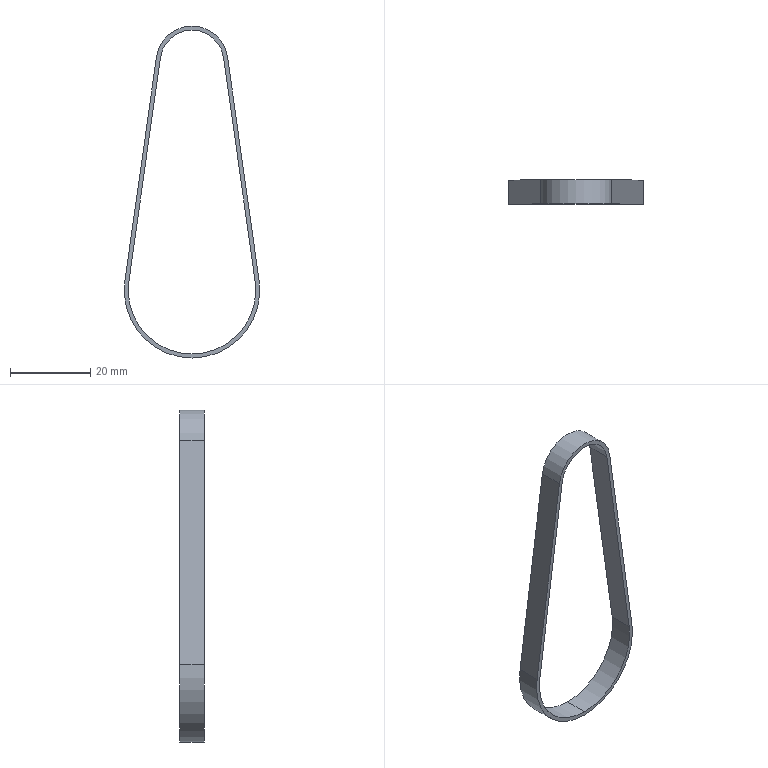Part | SolidWorks | features Extrusion 1 | 1 solid | 12 faces | box 33.828 x 6 x 82.868 mm | volume 1159 mm3 | cylinder 6 | plane 6 | commonest cylinder face diameters 31.828 x2 33.828 x2 15.908 x1 17.908 x1
STEP:
#1=CARTESIAN_POINT('',(15.758,6.,-54.778));
#2=VERTEX_POINT('',#1);
#3=CARTESIAN_POINT('',(0.,6.,-72.914));
#4=VERTEX_POINT('',#3);
#5=CARTESIAN_POINT('',(0.,6.,-57.));
#6=DIRECTION('',(0.,1.,0.));
#7=DIRECTION('',(0.,0.,1.));
#8=AXIS2_PLACEMENT_3D('',#5,#6,#7);
#9=CIRCLE('',#8,15.914);
#10=EDGE_CURVE('',#2,#4,#9,.T.);
#11=ORIENTED_EDGE('',*,*,#10,.T.);
#12=CARTESIAN_POINT('',(0.,0.,-72.914));
#13=VERTEX_POINT('',#12);
#14=CARTESIAN_POINT('',(0.,6.,-72.914));
#15=DIRECTION('',(0.,-1.,0.));
#16=VECTOR('',#15,1000.);
#17=LINE('',#14,#16);
#18=EDGE_CURVE('',#4,#13,#17,.T.);
#19=ORIENTED_EDGE('',*,*,#18,.T.);
#20=CARTESIAN_POINT('',(15.758,0.,-54.778));
#21=VERTEX_POINT('',#20);
#22=CARTESIAN_POINT('',(0.,0.,-57.));
#23=DIRECTION('',(0.,1.,0.));
#24=DIRECTION('',(0.,0.,1.));
#25=AXIS2_PLACEMENT_3D('',#22,#23,#24);
#26=CIRCLE('',#25,15.914);
#27=EDGE_CURVE('',#21,#13,#26,.T.);
#28=ORIENTED_EDGE('',*,*,#27,.F.);
#29=CARTESIAN_POINT('',(15.758,6.,-54.778));
#30=DIRECTION('',(0.,-1.,0.));
#31=VECTOR('',#30,1000.);
#32=LINE('',#29,#31);
#33=EDGE_CURVE('',#2,#21,#32,.T.);
#34=ORIENTED_EDGE('',*,*,#33,.F.);
#35=EDGE_LOOP('',(#11,#19,#28,#34));
#36=FACE_OUTER_BOUND('',#35,.T.);
#37=CARTESIAN_POINT('',(0.,6.,-57.));
#38=DIRECTION('',(0.,-1.,0.));
#39=DIRECTION('',(0.,0.,-1.));
#40=AXIS2_PLACEMENT_3D('',#37,#38,#39);
#41=CYLINDRICAL_SURFACE('',#40,15.914);
#42=ADVANCED_FACE('',(#36),#41,.F.);
#43=CARTESIAN_POINT('',(0.,6.,-73.914));
#44=VERTEX_POINT('',#43);
#45=CARTESIAN_POINT('',(-16.748,6.,-54.638));
#46=VERTEX_POINT('',#45);
#47=CARTESIAN_POINT('',(0.,6.,-57.));
#48=DIRECTION('',(0.,1.,0.));
#49=DIRECTION('',(0.,0.,1.));
#50=AXIS2_PLACEMENT_3D('',#47,#48,#49);
#51=CIRCLE('',#50,16.914);
#52=EDGE_CURVE('',#44,#46,#51,.T.);
#53=ORIENTED_EDGE('',*,*,#52,.F.);
#54=CARTESIAN_POINT('',(0.,0.,-73.914));
#55=VERTEX_POINT('',#54);
#56=CARTESIAN_POINT('',(0.,6.,-73.914));
#57=DIRECTION('',(0.,-1.,0.));
#58=VECTOR('',#57,1000.);
#59=LINE('',#56,#58);
#60=EDGE_CURVE('',#44,#55,#59,.T.);
#61=ORIENTED_EDGE('',*,*,#60,.T.);
#62=CARTESIAN_POINT('',(-16.748,0.,-54.638));
#63=VERTEX_POINT('',#62);
#64=CARTESIAN_POINT('',(0.,0.,-57.));
#65=DIRECTION('',(0.,1.,0.));
#66=DIRECTION('',(0.,0.,1.));
#67=AXIS2_PLACEMENT_3D('',#64,#65,#66);
#68=CIRCLE('',#67,16.914);
#69=EDGE_CURVE('',#55,#63,#68,.T.);
#70=ORIENTED_EDGE('',*,*,#69,.T.);
#71=CARTESIAN_POINT('',(-16.748,6.,-54.638));
#72=DIRECTION('',(0.,-1.,0.));
#73=VECTOR('',#72,1000.);
#74=LINE('',#71,#73);
#75=EDGE_CURVE('',#46,#63,#74,.T.);
#76=ORIENTED_EDGE('',*,*,#75,.F.);
#77=EDGE_LOOP('',(#53,#61,#70,#76));
#78=FACE_OUTER_BOUND('',#77,.T.);
#79=CARTESIAN_POINT('',(0.,6.,-57.));
#80=DIRECTION('',(0.,-1.,0.));
#81=DIRECTION('',(0.,0.,-1.));
#82=AXIS2_PLACEMENT_3D('',#79,#80,#81);
#83=CYLINDRICAL_SURFACE('',#82,16.914);
#84=ADVANCED_FACE('',(#78),#83,.T.);
#85=CARTESIAN_POINT('',(16.748,6.,-54.638));
#86=VERTEX_POINT('',#85);
#87=CARTESIAN_POINT('',(0.,6.,-57.));
#88=DIRECTION('',(0.,1.,0.));
#89=DIRECTION('',(0.,0.,1.));
#90=AXIS2_PLACEMENT_3D('',#87,#88,#89);
#91=CIRCLE('',#90,16.914);
#92=EDGE_CURVE('',#86,#44,#91,.T.);
#93=ORIENTED_EDGE('',*,*,#92,.T.);
#94=ORIENTED_EDGE('',*,*,#52,.T.);
#95=CARTESIAN_POINT('',(-8.866,6.,1.25));
#96=VERTEX_POINT('',#95);
#97=CARTESIAN_POINT('',(-16.748,6.,-54.638));
#98=DIRECTION('',(0.1396,0.,0.9902));
#99=VECTOR('',#98,1000.);
#100=LINE('',#97,#99);
#101=EDGE_CURVE('',#46,#96,#100,.T.);
#102=ORIENTED_EDGE('',*,*,#101,.T.);
#103=CARTESIAN_POINT('',(8.866,6.,1.25));
#104=VERTEX_POINT('',#103);
#105=CARTESIAN_POINT('',(0.,6.,0.));
#106=DIRECTION('',(0.,1.,0.));
#107=DIRECTION('',(0.,0.,1.));
#108=AXIS2_PLACEMENT_3D('',#105,#106,#107);
#109=CIRCLE('',#108,8.954);
#110=EDGE_CURVE('',#96,#104,#109,.T.);
#111=ORIENTED_EDGE('',*,*,#110,.T.);
#112=CARTESIAN_POINT('',(16.748,6.,-54.638));
#113=DIRECTION('',(0.1396,0.,-0.9902));
#114=VECTOR('',#113,1000.);
#115=LINE('',#112,#114);
#116=EDGE_CURVE('',#104,#86,#115,.T.);
#117=ORIENTED_EDGE('',*,*,#116,.T.);
#118=EDGE_LOOP('',(#93,#94,#102,#111,#117));
#119=FACE_OUTER_BOUND('',#118,.T.);
#120=CARTESIAN_POINT('',(7.876,6.,1.111));
#121=VERTEX_POINT('',#120);
#122=CARTESIAN_POINT('',(15.758,6.,-54.778));
#123=DIRECTION('',(0.1396,0.,-0.9902));
#124=VECTOR('',#123,1000.);
#125=LINE('',#122,#124);
#126=EDGE_CURVE('',#121,#2,#125,.T.);
#127=ORIENTED_EDGE('',*,*,#126,.F.);
#128=CARTESIAN_POINT('',(-7.876,6.,1.111));
#129=VERTEX_POINT('',#128);
#130=CARTESIAN_POINT('',(0.,6.,0.));
#131=DIRECTION('',(0.,1.,0.));
#132=DIRECTION('',(0.,0.,1.));
#133=AXIS2_PLACEMENT_3D('',#130,#131,#132);
#134=CIRCLE('',#133,7.954);
#135=EDGE_CURVE('',#129,#121,#134,.T.);
#136=ORIENTED_EDGE('',*,*,#135,.F.);
#137=CARTESIAN_POINT('',(-15.758,6.,-54.778));
#138=VERTEX_POINT('',#137);
#139=CARTESIAN_POINT('',(-15.758,6.,-54.778));
#140=DIRECTION('',(0.1396,0.,0.9902));
#141=VECTOR('',#140,1000.);
#142=LINE('',#139,#141);
#143=EDGE_CURVE('',#138,#129,#142,.T.);
#144=ORIENTED_EDGE('',*,*,#143,.F.);
#145=CARTESIAN_POINT('',(0.,6.,-57.));
#146=DIRECTION('',(0.,1.,0.));
#147=DIRECTION('',(0.,0.,1.));
#148=AXIS2_PLACEMENT_3D('',#145,#146,#147);
#149=CIRCLE('',#148,15.914);
#150=EDGE_CURVE('',#4,#138,#149,.T.);
#151=ORIENTED_EDGE('',*,*,#150,.F.);
#152=ORIENTED_EDGE('',*,*,#10,.F.);
#153=EDGE_LOOP('',(#127,#136,#144,#151,#152));
#154=FACE_BOUND('',#153,.T.);
#155=CARTESIAN_POINT('',(0.,6.,-57.));
#156=DIRECTION('',(0.,1.,0.));
#157=DIRECTION('',(0.,0.,1.));
#158=AXIS2_PLACEMENT_3D('',#155,#156,#157);
#159=PLANE('',#158);
#160=ADVANCED_FACE('',(#119,#154),#159,.T.);
#161=CARTESIAN_POINT('',(16.748,0.,-54.638));
#162=VERTEX_POINT('',#161);
#163=CARTESIAN_POINT('',(0.,0.,-57.));
#164=DIRECTION('',(0.,1.,0.));
#165=DIRECTION('',(0.,0.,1.));
#166=AXIS2_PLACEMENT_3D('',#163,#164,#165);
#167=CIRCLE('',#166,16.914);
#168=EDGE_CURVE('',#162,#55,#167,.T.);
#169=ORIENTED_EDGE('',*,*,#168,.F.);
#170=CARTESIAN_POINT('',(8.866,0.,1.25));
#171=VERTEX_POINT('',#170);
#172=CARTESIAN_POINT('',(16.748,0.,-54.638));
#173=DIRECTION('',(0.1396,0.,-0.9902));
#174=VECTOR('',#173,1000.);
#175=LINE('',#172,#174);
#176=EDGE_CURVE('',#171,#162,#175,.T.);
#177=ORIENTED_EDGE('',*,*,#176,.F.);
#178=CARTESIAN_POINT('',(-8.866,0.,1.25));
#179=VERTEX_POINT('',#178);
#180=CARTESIAN_POINT('',(0.,0.,0.));
#181=DIRECTION('',(0.,1.,0.));
#182=DIRECTION('',(0.,0.,1.));
#183=AXIS2_PLACEMENT_3D('',#180,#181,#182);
#184=CIRCLE('',#183,8.954);
#185=EDGE_CURVE('',#179,#171,#184,.T.);
#186=ORIENTED_EDGE('',*,*,#185,.F.);
#187=CARTESIAN_POINT('',(-16.748,0.,-54.638));
#188=DIRECTION('',(0.1396,0.,0.9902));
#189=VECTOR('',#188,1000.);
#190=LINE('',#187,#189);
#191=EDGE_CURVE('',#63,#179,#190,.T.);
#192=ORIENTED_EDGE('',*,*,#191,.F.);
#193=ORIENTED_EDGE('',*,*,#69,.F.);
#194=EDGE_LOOP('',(#169,#177,#186,#192,#193));
#195=FACE_OUTER_BOUND('',#194,.T.);
#196=CARTESIAN_POINT('',(-7.876,0.,1.111));
#197=VERTEX_POINT('',#196);
#198=CARTESIAN_POINT('',(7.876,0.,1.111));
#199=VERTEX_POINT('',#198);
#200=CARTESIAN_POINT('',(0.,0.,0.));
#201=DIRECTION('',(0.,1.,0.));
#202=DIRECTION('',(0.,0.,1.));
#203=AXIS2_PLACEMENT_3D('',#200,#201,#202);
#204=CIRCLE('',#203,7.954);
#205=EDGE_CURVE('',#197,#199,#204,.T.);
#206=ORIENTED_EDGE('',*,*,#205,.T.);
#207=CARTESIAN_POINT('',(15.758,0.,-54.778));
#208=DIRECTION('',(0.1396,0.,-0.9902));
#209=VECTOR('',#208,1000.);
#210=LINE('',#207,#209);
#211=EDGE_CURVE('',#199,#21,#210,.T.);
#212=ORIENTED_EDGE('',*,*,#211,.T.);
#213=ORIENTED_EDGE('',*,*,#27,.T.);
#214=CARTESIAN_POINT('',(-15.758,0.,-54.778));
#215=VERTEX_POINT('',#214);
#216=CARTESIAN_POINT('',(0.,0.,-57.));
#217=DIRECTION('',(0.,1.,0.));
#218=DIRECTION('',(0.,0.,1.));
#219=AXIS2_PLACEMENT_3D('',#216,#217,#218);
#220=CIRCLE('',#219,15.914);
#221=EDGE_CURVE('',#13,#215,#220,.T.);
#222=ORIENTED_EDGE('',*,*,#221,.T.);
#223=CARTESIAN_POINT('',(-15.758,0.,-54.778));
#224=DIRECTION('',(0.1396,0.,0.9902));
#225=VECTOR('',#224,1000.);
#226=LINE('',#223,#225);
#227=EDGE_CURVE('',#215,#197,#226,.T.);
#228=ORIENTED_EDGE('',*,*,#227,.T.);
#229=EDGE_LOOP('',(#206,#212,#213,#222,#228));
#230=FACE_BOUND('',#229,.T.);
#231=CARTESIAN_POINT('',(0.,0.,-57.));
#232=DIRECTION('',(0.,1.,0.));
#233=DIRECTION('',(0.,0.,1.));
#234=AXIS2_PLACEMENT_3D('',#231,#232,#233);
#235=PLANE('',#234);
#236=ADVANCED_FACE('',(#195,#230),#235,.F.);
#237=ORIENTED_EDGE('',*,*,#60,.F.);
#238=ORIENTED_EDGE('',*,*,#92,.F.);
#239=CARTESIAN_POINT('',(16.748,6.,-54.638));
#240=DIRECTION('',(0.,-1.,0.));
#241=VECTOR('',#240,1000.);
#242=LINE('',#239,#241);
#243=EDGE_CURVE('',#86,#162,#242,.T.);
#244=ORIENTED_EDGE('',*,*,#243,.T.);
#245=ORIENTED_EDGE('',*,*,#168,.T.);
#246=EDGE_LOOP('',(#237,#238,#244,#245));
#247=FACE_OUTER_BOUND('',#246,.T.);
#248=CARTESIAN_POINT('',(0.,6.,-57.));
#249=DIRECTION('',(0.,-1.,0.));
#250=DIRECTION('',(0.,0.,-1.));
#251=AXIS2_PLACEMENT_3D('',#248,#249,#250);
#252=CYLINDRICAL_SURFACE('',#251,16.914);
#253=ADVANCED_FACE('',(#247),#252,.T.);
#254=ORIENTED_EDGE('',*,*,#191,.T.);
#255=CARTESIAN_POINT('',(-8.866,6.,1.25));
#256=DIRECTION('',(0.,-1.,0.));
#257=VECTOR('',#256,1000.);
#258=LINE('',#255,#257);
#259=EDGE_CURVE('',#96,#179,#258,.T.);
#260=ORIENTED_EDGE('',*,*,#259,.F.);
#261=ORIENTED_EDGE('',*,*,#101,.F.);
#262=ORIENTED_EDGE('',*,*,#75,.T.);
#263=EDGE_LOOP('',(#254,#260,#261,#262));
#264=FACE_OUTER_BOUND('',#263,.T.);
#265=CARTESIAN_POINT('',(-16.748,6.,-54.638));
#266=DIRECTION('',(0.9902,0.,-0.1396));
#267=DIRECTION('',(-0.1396,0.,-0.9902));
#268=AXIS2_PLACEMENT_3D('',#265,#266,#267);
#269=PLANE('',#268);
#270=ADVANCED_FACE('',(#264),#269,.F.);
#271=ORIENTED_EDGE('',*,*,#185,.T.);
#272=CARTESIAN_POINT('',(8.866,6.,1.25));
#273=DIRECTION('',(0.,-1.,0.));
#274=VECTOR('',#273,1000.);
#275=LINE('',#272,#274);
#276=EDGE_CURVE('',#104,#171,#275,.T.);
#277=ORIENTED_EDGE('',*,*,#276,.F.);
#278=ORIENTED_EDGE('',*,*,#110,.F.);
#279=ORIENTED_EDGE('',*,*,#259,.T.);
#280=EDGE_LOOP('',(#271,#277,#278,#279));
#281=FACE_OUTER_BOUND('',#280,.T.);
#282=CARTESIAN_POINT('',(0.,6.,0.));
#283=DIRECTION('',(0.,-1.,0.));
#284=DIRECTION('',(0.,0.,-1.));
#285=AXIS2_PLACEMENT_3D('',#282,#283,#284);
#286=CYLINDRICAL_SURFACE('',#285,8.954);
#287=ADVANCED_FACE('',(#281),#286,.T.);
#288=ORIENTED_EDGE('',*,*,#176,.T.);
#289=ORIENTED_EDGE('',*,*,#243,.F.);
#290=ORIENTED_EDGE('',*,*,#116,.F.);
#291=ORIENTED_EDGE('',*,*,#276,.T.);
#292=EDGE_LOOP('',(#288,#289,#290,#291));
#293=FACE_OUTER_BOUND('',#292,.T.);
#294=CARTESIAN_POINT('',(16.748,6.,-54.638));
#295=DIRECTION('',(-0.9902,0.,-0.1396));
#296=DIRECTION('',(-0.1396,0.,0.9902));
#297=AXIS2_PLACEMENT_3D('',#294,#295,#296);
#298=PLANE('',#297);
#299=ADVANCED_FACE('',(#293),#298,.F.);
#300=ORIENTED_EDGE('',*,*,#205,.F.);
#301=CARTESIAN_POINT('',(-7.876,6.,1.111));
#302=DIRECTION('',(0.,-1.,0.));
#303=VECTOR('',#302,1000.);
#304=LINE('',#301,#303);
#305=EDGE_CURVE('',#129,#197,#304,.T.);
#306=ORIENTED_EDGE('',*,*,#305,.F.);
#307=ORIENTED_EDGE('',*,*,#135,.T.);
#308=CARTESIAN_POINT('',(7.876,6.,1.111));
#309=DIRECTION('',(0.,-1.,0.));
#310=VECTOR('',#309,1000.);
#311=LINE('',#308,#310);
#312=EDGE_CURVE('',#121,#199,#311,.T.);
#313=ORIENTED_EDGE('',*,*,#312,.T.);
#314=EDGE_LOOP('',(#300,#306,#307,#313));
#315=FACE_OUTER_BOUND('',#314,.T.);
#316=CARTESIAN_POINT('',(0.,6.,0.));
#317=DIRECTION('',(0.,-1.,0.));
#318=DIRECTION('',(0.,0.,-1.));
#319=AXIS2_PLACEMENT_3D('',#316,#317,#318);
#320=CYLINDRICAL_SURFACE('',#319,7.954);
#321=ADVANCED_FACE('',(#315),#320,.F.);
#322=ORIENTED_EDGE('',*,*,#211,.F.);
#323=ORIENTED_EDGE('',*,*,#312,.F.);
#324=ORIENTED_EDGE('',*,*,#126,.T.);
#325=ORIENTED_EDGE('',*,*,#33,.T.);
#326=EDGE_LOOP('',(#322,#323,#324,#325));
#327=FACE_OUTER_BOUND('',#326,.T.);
#328=CARTESIAN_POINT('',(15.758,6.,-54.778));
#329=DIRECTION('',(-0.9902,0.,-0.1396));
#330=DIRECTION('',(-0.1396,0.,0.9902));
#331=AXIS2_PLACEMENT_3D('',#328,#329,#330);
#332=PLANE('',#331);
#333=ADVANCED_FACE('',(#327),#332,.T.);
#334=ORIENTED_EDGE('',*,*,#18,.F.);
#335=ORIENTED_EDGE('',*,*,#150,.T.);
#336=CARTESIAN_POINT('',(-15.758,6.,-54.778));
#337=DIRECTION('',(0.,-1.,0.));
#338=VECTOR('',#337,1000.);
#339=LINE('',#336,#338);
#340=EDGE_CURVE('',#138,#215,#339,.T.);
#341=ORIENTED_EDGE('',*,*,#340,.T.);
#342=ORIENTED_EDGE('',*,*,#221,.F.);
#343=EDGE_LOOP('',(#334,#335,#341,#342));
#344=FACE_OUTER_BOUND('',#343,.T.);
#345=CARTESIAN_POINT('',(0.,6.,-57.));
#346=DIRECTION('',(0.,-1.,0.));
#347=DIRECTION('',(0.,0.,-1.));
#348=AXIS2_PLACEMENT_3D('',#345,#346,#347);
#349=CYLINDRICAL_SURFACE('',#348,15.914);
#350=ADVANCED_FACE('',(#344),#349,.F.);
#351=ORIENTED_EDGE('',*,*,#227,.F.);
#352=ORIENTED_EDGE('',*,*,#340,.F.);
#353=ORIENTED_EDGE('',*,*,#143,.T.);
#354=ORIENTED_EDGE('',*,*,#305,.T.);
#355=EDGE_LOOP('',(#351,#352,#353,#354));
#356=FACE_OUTER_BOUND('',#355,.T.);
#357=CARTESIAN_POINT('',(-15.758,6.,-54.778));
#358=DIRECTION('',(0.9902,0.,-0.1396));
#359=DIRECTION('',(-0.1396,0.,-0.9902));
#360=AXIS2_PLACEMENT_3D('',#357,#358,#359);
#361=PLANE('',#360);
#362=ADVANCED_FACE('',(#356),#361,.T.);
#363=CLOSED_SHELL('',(#42,#84,#160,#236,#253,#270,#287,#299,#321,#333,#350,#362));
#364=MANIFOLD_SOLID_BREP('',#363);
#365=CARTESIAN_POINT('',(0.,0.,0.));
#366=DIRECTION('',(0.,0.,1.));
#367=DIRECTION('',(1.,0.,0.));
#368=AXIS2_PLACEMENT_3D('',#365,#366,#367);
#369=(LENGTH_UNIT()NAMED_UNIT(*)SI_UNIT(.MILLI.,.METRE.));
#370=UNCERTAINTY_MEASURE_WITH_UNIT(LENGTH_MEASURE(0.00001),#369,'','');
#371=(NAMED_UNIT(*)PLANE_ANGLE_UNIT()SI_UNIT($,.RADIAN.));
#372=(NAMED_UNIT(*)SI_UNIT($,.STERADIAN.)SOLID_ANGLE_UNIT());
#373=(GEOMETRIC_REPRESENTATION_CONTEXT(3)GLOBAL_UNCERTAINTY_ASSIGNED_CONTEXT((#370))GLOBAL_UNIT_ASSIGNED_CONTEXT((#369,#371,#372))REPRESENTATION_CONTEXT('',''));
#374=ADVANCED_BREP_SHAPE_REPRESENTATION('',(#364,#368),#373);